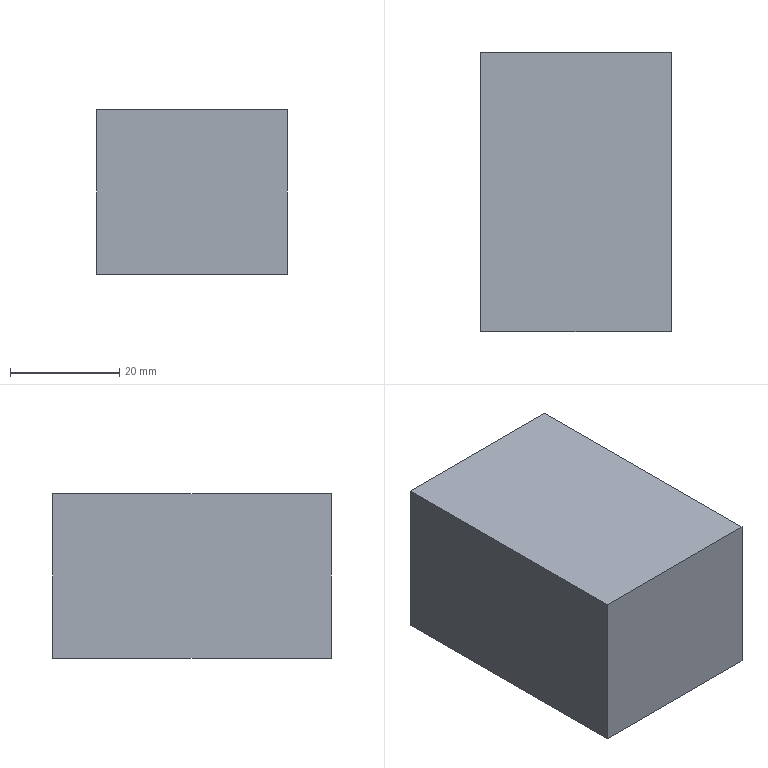Part | SolidWorks | features Extrusion 1 | 1 solid | 6 faces | box 34.866 x 50.94 x 30 mm | volume 53282 mm3 | plane 6
STEP:
#1=CARTESIAN_POINT('',(17.433,-25.47,0.));
#2=VERTEX_POINT('',#1);
#3=CARTESIAN_POINT('',(17.433,25.47,0.));
#4=VERTEX_POINT('',#3);
#5=CARTESIAN_POINT('',(17.433,25.47,0.));
#6=DIRECTION('',(0.,1.,0.));
#7=VECTOR('',#6,1000.);
#8=LINE('',#5,#7);
#9=EDGE_CURVE('',#2,#4,#8,.T.);
#10=ORIENTED_EDGE('',*,*,#9,.F.);
#11=CARTESIAN_POINT('',(17.433,-25.47,-30.));
#12=VERTEX_POINT('',#11);
#13=CARTESIAN_POINT('',(17.433,-25.47,-30.));
#14=DIRECTION('',(0.,0.,1.));
#15=VECTOR('',#14,1000.);
#16=LINE('',#13,#15);
#17=EDGE_CURVE('',#12,#2,#16,.T.);
#18=ORIENTED_EDGE('',*,*,#17,.F.);
#19=CARTESIAN_POINT('',(17.433,25.47,-30.));
#20=VERTEX_POINT('',#19);
#21=CARTESIAN_POINT('',(17.433,25.47,-30.));
#22=DIRECTION('',(0.,1.,0.));
#23=VECTOR('',#22,1000.);
#24=LINE('',#21,#23);
#25=EDGE_CURVE('',#12,#20,#24,.T.);
#26=ORIENTED_EDGE('',*,*,#25,.T.);
#27=CARTESIAN_POINT('',(17.433,25.47,-30.));
#28=DIRECTION('',(0.,0.,1.));
#29=VECTOR('',#28,1000.);
#30=LINE('',#27,#29);
#31=EDGE_CURVE('',#20,#4,#30,.T.);
#32=ORIENTED_EDGE('',*,*,#31,.T.);
#33=EDGE_LOOP('',(#10,#18,#26,#32));
#34=FACE_OUTER_BOUND('',#33,.T.);
#35=CARTESIAN_POINT('',(17.433,25.47,-30.));
#36=DIRECTION('',(1.,0.,0.));
#37=DIRECTION('',(0.,1.,0.));
#38=AXIS2_PLACEMENT_3D('',#35,#36,#37);
#39=PLANE('',#38);
#40=ADVANCED_FACE('',(#34),#39,.T.);
#41=CARTESIAN_POINT('',(-17.433,-25.47,0.));
#42=VERTEX_POINT('',#41);
#43=CARTESIAN_POINT('',(-17.433,-25.47,0.));
#44=DIRECTION('',(1.,0.,0.));
#45=VECTOR('',#44,1000.);
#46=LINE('',#43,#45);
#47=EDGE_CURVE('',#42,#2,#46,.T.);
#48=ORIENTED_EDGE('',*,*,#47,.F.);
#49=CARTESIAN_POINT('',(-17.433,-25.47,-30.));
#50=VERTEX_POINT('',#49);
#51=CARTESIAN_POINT('',(-17.433,-25.47,-30.));
#52=DIRECTION('',(0.,0.,1.));
#53=VECTOR('',#52,1000.);
#54=LINE('',#51,#53);
#55=EDGE_CURVE('',#50,#42,#54,.T.);
#56=ORIENTED_EDGE('',*,*,#55,.F.);
#57=CARTESIAN_POINT('',(-17.433,-25.47,-30.));
#58=DIRECTION('',(1.,0.,0.));
#59=VECTOR('',#58,1000.);
#60=LINE('',#57,#59);
#61=EDGE_CURVE('',#50,#12,#60,.T.);
#62=ORIENTED_EDGE('',*,*,#61,.T.);
#63=ORIENTED_EDGE('',*,*,#17,.T.);
#64=EDGE_LOOP('',(#48,#56,#62,#63));
#65=FACE_OUTER_BOUND('',#64,.T.);
#66=CARTESIAN_POINT('',(-17.433,-25.47,-30.));
#67=DIRECTION('',(0.,-1.,0.));
#68=DIRECTION('',(0.,0.,-1.));
#69=AXIS2_PLACEMENT_3D('',#66,#67,#68);
#70=PLANE('',#69);
#71=ADVANCED_FACE('',(#65),#70,.T.);
#72=CARTESIAN_POINT('',(-17.433,25.47,0.));
#73=VERTEX_POINT('',#72);
#74=CARTESIAN_POINT('',(-17.433,25.47,0.));
#75=DIRECTION('',(0.,-1.,0.));
#76=VECTOR('',#75,1000.);
#77=LINE('',#74,#76);
#78=EDGE_CURVE('',#73,#42,#77,.T.);
#79=ORIENTED_EDGE('',*,*,#78,.F.);
#80=CARTESIAN_POINT('',(-17.433,25.47,-30.));
#81=VERTEX_POINT('',#80);
#82=CARTESIAN_POINT('',(-17.433,25.47,-30.));
#83=DIRECTION('',(0.,0.,1.));
#84=VECTOR('',#83,1000.);
#85=LINE('',#82,#84);
#86=EDGE_CURVE('',#81,#73,#85,.T.);
#87=ORIENTED_EDGE('',*,*,#86,.F.);
#88=CARTESIAN_POINT('',(-17.433,25.47,-30.));
#89=DIRECTION('',(0.,-1.,0.));
#90=VECTOR('',#89,1000.);
#91=LINE('',#88,#90);
#92=EDGE_CURVE('',#81,#50,#91,.T.);
#93=ORIENTED_EDGE('',*,*,#92,.T.);
#94=ORIENTED_EDGE('',*,*,#55,.T.);
#95=EDGE_LOOP('',(#79,#87,#93,#94));
#96=FACE_OUTER_BOUND('',#95,.T.);
#97=CARTESIAN_POINT('',(-17.433,25.47,-30.));
#98=DIRECTION('',(-1.,0.,0.));
#99=DIRECTION('',(0.,0.,1.));
#100=AXIS2_PLACEMENT_3D('',#97,#98,#99);
#101=PLANE('',#100);
#102=ADVANCED_FACE('',(#96),#101,.T.);
#103=CARTESIAN_POINT('',(-17.433,25.47,0.));
#104=DIRECTION('',(-1.,0.,0.));
#105=VECTOR('',#104,1000.);
#106=LINE('',#103,#105);
#107=EDGE_CURVE('',#4,#73,#106,.T.);
#108=ORIENTED_EDGE('',*,*,#107,.F.);
#109=ORIENTED_EDGE('',*,*,#31,.F.);
#110=CARTESIAN_POINT('',(-17.433,25.47,-30.));
#111=DIRECTION('',(-1.,0.,0.));
#112=VECTOR('',#111,1000.);
#113=LINE('',#110,#112);
#114=EDGE_CURVE('',#20,#81,#113,.T.);
#115=ORIENTED_EDGE('',*,*,#114,.T.);
#116=ORIENTED_EDGE('',*,*,#86,.T.);
#117=EDGE_LOOP('',(#108,#109,#115,#116));
#118=FACE_OUTER_BOUND('',#117,.T.);
#119=CARTESIAN_POINT('',(-17.433,25.47,-30.));
#120=DIRECTION('',(0.,1.,0.));
#121=DIRECTION('',(0.,0.,1.));
#122=AXIS2_PLACEMENT_3D('',#119,#120,#121);
#123=PLANE('',#122);
#124=ADVANCED_FACE('',(#118),#123,.T.);
#125=ORIENTED_EDGE('',*,*,#25,.F.);
#126=ORIENTED_EDGE('',*,*,#61,.F.);
#127=ORIENTED_EDGE('',*,*,#92,.F.);
#128=ORIENTED_EDGE('',*,*,#114,.F.);
#129=EDGE_LOOP('',(#125,#126,#127,#128));
#130=FACE_OUTER_BOUND('',#129,.T.);
#131=CARTESIAN_POINT('',(0.,0.,-30.));
#132=DIRECTION('',(0.,0.,1.));
#133=DIRECTION('',(1.,0.,0.));
#134=AXIS2_PLACEMENT_3D('',#131,#132,#133);
#135=PLANE('',#134);
#136=ADVANCED_FACE('',(#130),#135,.F.);
#137=ORIENTED_EDGE('',*,*,#9,.T.);
#138=ORIENTED_EDGE('',*,*,#107,.T.);
#139=ORIENTED_EDGE('',*,*,#78,.T.);
#140=ORIENTED_EDGE('',*,*,#47,.T.);
#141=EDGE_LOOP('',(#137,#138,#139,#140));
#142=FACE_OUTER_BOUND('',#141,.T.);
#143=CARTESIAN_POINT('',(0.,0.,0.));
#144=DIRECTION('',(0.,0.,1.));
#145=DIRECTION('',(1.,0.,0.));
#146=AXIS2_PLACEMENT_3D('',#143,#144,#145);
#147=PLANE('',#146);
#148=ADVANCED_FACE('',(#142),#147,.T.);
#149=CLOSED_SHELL('',(#40,#71,#102,#124,#136,#148));
#150=MANIFOLD_SOLID_BREP('',#149);
#151=CARTESIAN_POINT('',(0.,0.,0.));
#152=DIRECTION('',(0.,0.,1.));
#153=DIRECTION('',(1.,0.,0.));
#154=AXIS2_PLACEMENT_3D('',#151,#152,#153);
#155=(LENGTH_UNIT()NAMED_UNIT(*)SI_UNIT(.MILLI.,.METRE.));
#156=UNCERTAINTY_MEASURE_WITH_UNIT(LENGTH_MEASURE(0.00001),#155,'','');
#157=(NAMED_UNIT(*)PLANE_ANGLE_UNIT()SI_UNIT($,.RADIAN.));
#158=(NAMED_UNIT(*)SI_UNIT($,.STERADIAN.)SOLID_ANGLE_UNIT());
#159=(GEOMETRIC_REPRESENTATION_CONTEXT(3)GLOBAL_UNCERTAINTY_ASSIGNED_CONTEXT((#156))GLOBAL_UNIT_ASSIGNED_CONTEXT((#155,#157,#158))REPRESENTATION_CONTEXT('',''));
#160=ADVANCED_BREP_SHAPE_REPRESENTATION('',(#150,#154),#159);